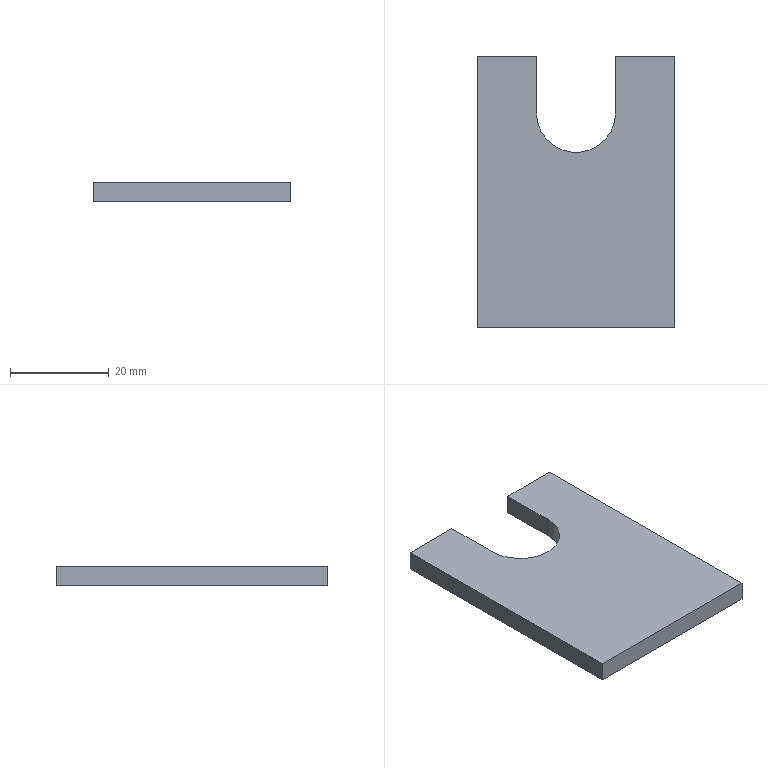Part | STEP file | Station 3 cylinder connecting plate | 1 solid | 10 faces | box 40 x 55 x 4 mm | volume 7662 mm3 | plane 9 | cylinder 1 | commonest cylinder face diameters 16 x1
STEP:
#1=CARTESIAN_POINT('',(20.,27.5,-2.));
#2=VERTEX_POINT('',#1);
#3=CARTESIAN_POINT('',(8.,27.5,-2.));
#4=VERTEX_POINT('',#3);
#5=CARTESIAN_POINT('',(8.,27.5,-2.));
#6=DIRECTION('',(-1.,0.,0.));
#7=VECTOR('',#6,1000.);
#8=LINE('',#5,#7);
#9=EDGE_CURVE('',#2,#4,#8,.T.);
#10=ORIENTED_EDGE('',*,*,#9,.T.);
#11=CARTESIAN_POINT('',(8.,27.5,2.));
#12=VERTEX_POINT('',#11);
#13=CARTESIAN_POINT('',(8.,27.5,2.));
#14=DIRECTION('',(0.,0.,-1.));
#15=VECTOR('',#14,1000.);
#16=LINE('',#13,#15);
#17=EDGE_CURVE('',#12,#4,#16,.T.);
#18=ORIENTED_EDGE('',*,*,#17,.F.);
#19=CARTESIAN_POINT('',(20.,27.5,2.));
#20=VERTEX_POINT('',#19);
#21=CARTESIAN_POINT('',(8.,27.5,2.));
#22=DIRECTION('',(-1.,0.,0.));
#23=VECTOR('',#22,1000.);
#24=LINE('',#21,#23);
#25=EDGE_CURVE('',#20,#12,#24,.T.);
#26=ORIENTED_EDGE('',*,*,#25,.F.);
#27=CARTESIAN_POINT('',(20.,27.5,2.));
#28=DIRECTION('',(0.,0.,-1.));
#29=VECTOR('',#28,1000.);
#30=LINE('',#27,#29);
#31=EDGE_CURVE('',#20,#2,#30,.T.);
#32=ORIENTED_EDGE('',*,*,#31,.T.);
#33=EDGE_LOOP('',(#10,#18,#26,#32));
#34=FACE_OUTER_BOUND('',#33,.T.);
#35=CARTESIAN_POINT('',(8.,27.5,2.));
#36=DIRECTION('',(0.,-1.,0.));
#37=DIRECTION('',(0.,0.,-1.));
#38=AXIS2_PLACEMENT_3D('',#35,#36,#37);
#39=PLANE('',#38);
#40=ADVANCED_FACE('',(#34),#39,.F.);
#41=CARTESIAN_POINT('',(8.,16.,-2.));
#42=VERTEX_POINT('',#41);
#43=CARTESIAN_POINT('',(8.,27.5,-2.));
#44=DIRECTION('',(0.,-1.,0.));
#45=VECTOR('',#44,1000.);
#46=LINE('',#43,#45);
#47=EDGE_CURVE('',#4,#42,#46,.T.);
#48=ORIENTED_EDGE('',*,*,#47,.T.);
#49=CARTESIAN_POINT('',(8.,16.,2.));
#50=VERTEX_POINT('',#49);
#51=CARTESIAN_POINT('',(8.,16.,2.));
#52=DIRECTION('',(0.,0.,-1.));
#53=VECTOR('',#52,1000.);
#54=LINE('',#51,#53);
#55=EDGE_CURVE('',#50,#42,#54,.T.);
#56=ORIENTED_EDGE('',*,*,#55,.F.);
#57=CARTESIAN_POINT('',(8.,27.5,2.));
#58=DIRECTION('',(0.,-1.,0.));
#59=VECTOR('',#58,1000.);
#60=LINE('',#57,#59);
#61=EDGE_CURVE('',#12,#50,#60,.T.);
#62=ORIENTED_EDGE('',*,*,#61,.F.);
#63=ORIENTED_EDGE('',*,*,#17,.T.);
#64=EDGE_LOOP('',(#48,#56,#62,#63));
#65=FACE_OUTER_BOUND('',#64,.T.);
#66=CARTESIAN_POINT('',(8.,27.5,2.));
#67=DIRECTION('',(1.,0.,0.));
#68=DIRECTION('',(0.,1.,0.));
#69=AXIS2_PLACEMENT_3D('',#66,#67,#68);
#70=PLANE('',#69);
#71=ADVANCED_FACE('',(#65),#70,.F.);
#72=CARTESIAN_POINT('',(-8.,16.,-2.));
#73=VERTEX_POINT('',#72);
#74=CARTESIAN_POINT('',(0.,16.,-2.));
#75=DIRECTION('',(0.,0.,-1.));
#76=DIRECTION('',(1.,0.,0.));
#77=AXIS2_PLACEMENT_3D('',#74,#75,#76);
#78=CIRCLE('',#77,8.);
#79=EDGE_CURVE('',#42,#73,#78,.T.);
#80=ORIENTED_EDGE('',*,*,#79,.T.);
#81=CARTESIAN_POINT('',(-8.,16.,2.));
#82=VERTEX_POINT('',#81);
#83=CARTESIAN_POINT('',(-8.,16.,2.));
#84=DIRECTION('',(0.,0.,-1.));
#85=VECTOR('',#84,1000.);
#86=LINE('',#83,#85);
#87=EDGE_CURVE('',#82,#73,#86,.T.);
#88=ORIENTED_EDGE('',*,*,#87,.F.);
#89=CARTESIAN_POINT('',(0.,16.,2.));
#90=DIRECTION('',(0.,0.,-1.));
#91=DIRECTION('',(1.,0.,0.));
#92=AXIS2_PLACEMENT_3D('',#89,#90,#91);
#93=CIRCLE('',#92,8.);
#94=EDGE_CURVE('',#50,#82,#93,.T.);
#95=ORIENTED_EDGE('',*,*,#94,.F.);
#96=ORIENTED_EDGE('',*,*,#55,.T.);
#97=EDGE_LOOP('',(#80,#88,#95,#96));
#98=FACE_OUTER_BOUND('',#97,.T.);
#99=CARTESIAN_POINT('',(0.,16.,2.));
#100=DIRECTION('',(0.,0.,-1.));
#101=DIRECTION('',(-1.,0.,0.));
#102=AXIS2_PLACEMENT_3D('',#99,#100,#101);
#103=CYLINDRICAL_SURFACE('',#102,8.);
#104=ADVANCED_FACE('',(#98),#103,.F.);
#105=CARTESIAN_POINT('',(-8.,27.5,-2.));
#106=VERTEX_POINT('',#105);
#107=CARTESIAN_POINT('',(-8.,16.,-2.));
#108=DIRECTION('',(0.,1.,0.));
#109=VECTOR('',#108,1000.);
#110=LINE('',#107,#109);
#111=EDGE_CURVE('',#73,#106,#110,.T.);
#112=ORIENTED_EDGE('',*,*,#111,.T.);
#113=CARTESIAN_POINT('',(-8.,27.5,2.));
#114=VERTEX_POINT('',#113);
#115=CARTESIAN_POINT('',(-8.,27.5,2.));
#116=DIRECTION('',(0.,0.,-1.));
#117=VECTOR('',#116,1000.);
#118=LINE('',#115,#117);
#119=EDGE_CURVE('',#114,#106,#118,.T.);
#120=ORIENTED_EDGE('',*,*,#119,.F.);
#121=CARTESIAN_POINT('',(-8.,16.,2.));
#122=DIRECTION('',(0.,1.,0.));
#123=VECTOR('',#122,1000.);
#124=LINE('',#121,#123);
#125=EDGE_CURVE('',#82,#114,#124,.T.);
#126=ORIENTED_EDGE('',*,*,#125,.F.);
#127=ORIENTED_EDGE('',*,*,#87,.T.);
#128=EDGE_LOOP('',(#112,#120,#126,#127));
#129=FACE_OUTER_BOUND('',#128,.T.);
#130=CARTESIAN_POINT('',(-8.,16.,2.));
#131=DIRECTION('',(-1.,0.,0.));
#132=DIRECTION('',(0.,0.,1.));
#133=AXIS2_PLACEMENT_3D('',#130,#131,#132);
#134=PLANE('',#133);
#135=ADVANCED_FACE('',(#129),#134,.F.);
#136=CARTESIAN_POINT('',(-20.,27.5,-2.));
#137=VERTEX_POINT('',#136);
#138=CARTESIAN_POINT('',(-20.,27.5,-2.));
#139=DIRECTION('',(-1.,0.,0.));
#140=VECTOR('',#139,1000.);
#141=LINE('',#138,#140);
#142=EDGE_CURVE('',#106,#137,#141,.T.);
#143=ORIENTED_EDGE('',*,*,#142,.T.);
#144=CARTESIAN_POINT('',(-20.,27.5,2.));
#145=VERTEX_POINT('',#144);
#146=CARTESIAN_POINT('',(-20.,27.5,2.));
#147=DIRECTION('',(0.,0.,-1.));
#148=VECTOR('',#147,1000.);
#149=LINE('',#146,#148);
#150=EDGE_CURVE('',#145,#137,#149,.T.);
#151=ORIENTED_EDGE('',*,*,#150,.F.);
#152=CARTESIAN_POINT('',(-20.,27.5,2.));
#153=DIRECTION('',(-1.,0.,0.));
#154=VECTOR('',#153,1000.);
#155=LINE('',#152,#154);
#156=EDGE_CURVE('',#114,#145,#155,.T.);
#157=ORIENTED_EDGE('',*,*,#156,.F.);
#158=ORIENTED_EDGE('',*,*,#119,.T.);
#159=EDGE_LOOP('',(#143,#151,#157,#158));
#160=FACE_OUTER_BOUND('',#159,.T.);
#161=CARTESIAN_POINT('',(-20.,27.5,2.));
#162=DIRECTION('',(0.,-1.,0.));
#163=DIRECTION('',(0.,0.,-1.));
#164=AXIS2_PLACEMENT_3D('',#161,#162,#163);
#165=PLANE('',#164);
#166=ADVANCED_FACE('',(#160),#165,.F.);
#167=CARTESIAN_POINT('',(-20.,-27.5,-2.));
#168=VERTEX_POINT('',#167);
#169=CARTESIAN_POINT('',(-20.,-27.5,-2.));
#170=DIRECTION('',(0.,-1.,0.));
#171=VECTOR('',#170,1000.);
#172=LINE('',#169,#171);
#173=EDGE_CURVE('',#137,#168,#172,.T.);
#174=ORIENTED_EDGE('',*,*,#173,.T.);
#175=CARTESIAN_POINT('',(-20.,-27.5,2.));
#176=VERTEX_POINT('',#175);
#177=CARTESIAN_POINT('',(-20.,-27.5,2.));
#178=DIRECTION('',(0.,0.,-1.));
#179=VECTOR('',#178,1000.);
#180=LINE('',#177,#179);
#181=EDGE_CURVE('',#176,#168,#180,.T.);
#182=ORIENTED_EDGE('',*,*,#181,.F.);
#183=CARTESIAN_POINT('',(-20.,-27.5,2.));
#184=DIRECTION('',(0.,-1.,0.));
#185=VECTOR('',#184,1000.);
#186=LINE('',#183,#185);
#187=EDGE_CURVE('',#145,#176,#186,.T.);
#188=ORIENTED_EDGE('',*,*,#187,.F.);
#189=ORIENTED_EDGE('',*,*,#150,.T.);
#190=EDGE_LOOP('',(#174,#182,#188,#189));
#191=FACE_OUTER_BOUND('',#190,.T.);
#192=CARTESIAN_POINT('',(-20.,-27.5,2.));
#193=DIRECTION('',(1.,0.,0.));
#194=DIRECTION('',(0.,0.,-1.));
#195=AXIS2_PLACEMENT_3D('',#192,#193,#194);
#196=PLANE('',#195);
#197=ADVANCED_FACE('',(#191),#196,.F.);
#198=CARTESIAN_POINT('',(20.,-27.5,-2.));
#199=VERTEX_POINT('',#198);
#200=CARTESIAN_POINT('',(-20.,-27.5,-2.));
#201=DIRECTION('',(1.,0.,0.));
#202=VECTOR('',#201,1000.);
#203=LINE('',#200,#202);
#204=EDGE_CURVE('',#168,#199,#203,.T.);
#205=ORIENTED_EDGE('',*,*,#204,.T.);
#206=CARTESIAN_POINT('',(20.,-27.5,2.));
#207=VERTEX_POINT('',#206);
#208=CARTESIAN_POINT('',(20.,-27.5,2.));
#209=DIRECTION('',(0.,0.,-1.));
#210=VECTOR('',#209,1000.);
#211=LINE('',#208,#210);
#212=EDGE_CURVE('',#207,#199,#211,.T.);
#213=ORIENTED_EDGE('',*,*,#212,.F.);
#214=CARTESIAN_POINT('',(-20.,-27.5,2.));
#215=DIRECTION('',(1.,0.,0.));
#216=VECTOR('',#215,1000.);
#217=LINE('',#214,#216);
#218=EDGE_CURVE('',#176,#207,#217,.T.);
#219=ORIENTED_EDGE('',*,*,#218,.F.);
#220=ORIENTED_EDGE('',*,*,#181,.T.);
#221=EDGE_LOOP('',(#205,#213,#219,#220));
#222=FACE_OUTER_BOUND('',#221,.T.);
#223=CARTESIAN_POINT('',(-20.,-27.5,2.));
#224=DIRECTION('',(0.,1.,0.));
#225=DIRECTION('',(0.,0.,1.));
#226=AXIS2_PLACEMENT_3D('',#223,#224,#225);
#227=PLANE('',#226);
#228=ADVANCED_FACE('',(#222),#227,.F.);
#229=CARTESIAN_POINT('',(20.,-27.5,-2.));
#230=DIRECTION('',(0.,1.,0.));
#231=VECTOR('',#230,1000.);
#232=LINE('',#229,#231);
#233=EDGE_CURVE('',#199,#2,#232,.T.);
#234=ORIENTED_EDGE('',*,*,#233,.T.);
#235=ORIENTED_EDGE('',*,*,#31,.F.);
#236=CARTESIAN_POINT('',(20.,-27.5,2.));
#237=DIRECTION('',(0.,1.,0.));
#238=VECTOR('',#237,1000.);
#239=LINE('',#236,#238);
#240=EDGE_CURVE('',#207,#20,#239,.T.);
#241=ORIENTED_EDGE('',*,*,#240,.F.);
#242=ORIENTED_EDGE('',*,*,#212,.T.);
#243=EDGE_LOOP('',(#234,#235,#241,#242));
#244=FACE_OUTER_BOUND('',#243,.T.);
#245=CARTESIAN_POINT('',(20.,-27.5,2.));
#246=DIRECTION('',(-1.,0.,0.));
#247=DIRECTION('',(0.,0.,1.));
#248=AXIS2_PLACEMENT_3D('',#245,#246,#247);
#249=PLANE('',#248);
#250=ADVANCED_FACE('',(#244),#249,.F.);
#251=ORIENTED_EDGE('',*,*,#25,.T.);
#252=ORIENTED_EDGE('',*,*,#61,.T.);
#253=ORIENTED_EDGE('',*,*,#94,.T.);
#254=ORIENTED_EDGE('',*,*,#125,.T.);
#255=ORIENTED_EDGE('',*,*,#156,.T.);
#256=ORIENTED_EDGE('',*,*,#187,.T.);
#257=ORIENTED_EDGE('',*,*,#218,.T.);
#258=ORIENTED_EDGE('',*,*,#240,.T.);
#259=EDGE_LOOP('',(#251,#252,#253,#254,#255,#256,#257,#258));
#260=FACE_OUTER_BOUND('',#259,.T.);
#261=CARTESIAN_POINT('',(0.,16.,2.));
#262=DIRECTION('',(0.,0.,1.));
#263=DIRECTION('',(1.,0.,0.));
#264=AXIS2_PLACEMENT_3D('',#261,#262,#263);
#265=PLANE('',#264);
#266=ADVANCED_FACE('',(#260),#265,.T.);
#267=ORIENTED_EDGE('',*,*,#9,.F.);
#268=ORIENTED_EDGE('',*,*,#233,.F.);
#269=ORIENTED_EDGE('',*,*,#204,.F.);
#270=ORIENTED_EDGE('',*,*,#173,.F.);
#271=ORIENTED_EDGE('',*,*,#142,.F.);
#272=ORIENTED_EDGE('',*,*,#111,.F.);
#273=ORIENTED_EDGE('',*,*,#79,.F.);
#274=ORIENTED_EDGE('',*,*,#47,.F.);
#275=EDGE_LOOP('',(#267,#268,#269,#270,#271,#272,#273,#274));
#276=FACE_OUTER_BOUND('',#275,.T.);
#277=CARTESIAN_POINT('',(0.,16.,-2.));
#278=DIRECTION('',(0.,0.,1.));
#279=DIRECTION('',(1.,0.,0.));
#280=AXIS2_PLACEMENT_3D('',#277,#278,#279);
#281=PLANE('',#280);
#282=ADVANCED_FACE('',(#276),#281,.F.);
#283=CLOSED_SHELL('',(#40,#71,#104,#135,#166,#197,#228,#250,#266,#282));
#284=MANIFOLD_SOLID_BREP('',#283);
#285=CARTESIAN_POINT('',(0.,0.,0.));
#286=DIRECTION('',(0.,0.,1.));
#287=DIRECTION('',(1.,0.,0.));
#288=AXIS2_PLACEMENT_3D('',#285,#286,#287);
#289=(LENGTH_UNIT()NAMED_UNIT(*)SI_UNIT(.MILLI.,.METRE.));
#290=UNCERTAINTY_MEASURE_WITH_UNIT(LENGTH_MEASURE(0.00001),#289,'','');
#291=(NAMED_UNIT(*)PLANE_ANGLE_UNIT()SI_UNIT($,.RADIAN.));
#292=(NAMED_UNIT(*)SI_UNIT($,.STERADIAN.)SOLID_ANGLE_UNIT());
#293=(GEOMETRIC_REPRESENTATION_CONTEXT(3)GLOBAL_UNCERTAINTY_ASSIGNED_CONTEXT((#290))GLOBAL_UNIT_ASSIGNED_CONTEXT((#289,#291,#292))REPRESENTATION_CONTEXT('',''));
#294=ADVANCED_BREP_SHAPE_REPRESENTATION('',(#284,#288),#293);